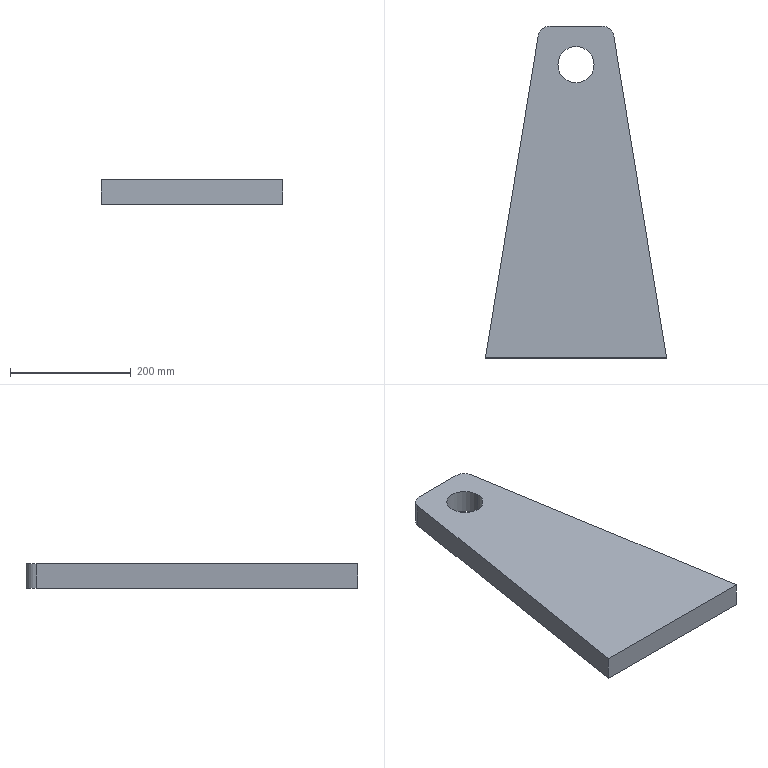Part | SolidWorks | features Extrusion 1 | 1 solid | 10 faces | box 300 x 550 x 40 mm | volume 4502251 mm3 | plane 6 | cylinder 4 | commonest cylinder face diameters 40 x2 60 x2
STEP:
#1=CARTESIAN_POINT('',(120.,486.,40.));
#2=VERTEX_POINT('',#1);
#3=CARTESIAN_POINT('',(180.,486.,40.));
#4=VERTEX_POINT('',#3);
#5=CARTESIAN_POINT('',(150.,486.,40.));
#6=DIRECTION('',(0.,0.,1.));
#7=DIRECTION('',(1.,0.,0.));
#8=AXIS2_PLACEMENT_3D('',#5,#6,#7);
#9=CIRCLE('',#8,30.);
#10=EDGE_CURVE('',#2,#4,#9,.T.);
#11=ORIENTED_EDGE('',*,*,#10,.T.);
#12=CARTESIAN_POINT('',(180.,486.,0.));
#13=VERTEX_POINT('',#12);
#14=CARTESIAN_POINT('',(180.,486.,40.));
#15=DIRECTION('',(0.,0.,-1.));
#16=VECTOR('',#15,1000.);
#17=LINE('',#14,#16);
#18=EDGE_CURVE('',#4,#13,#17,.T.);
#19=ORIENTED_EDGE('',*,*,#18,.T.);
#20=CARTESIAN_POINT('',(120.,486.,0.));
#21=VERTEX_POINT('',#20);
#22=CARTESIAN_POINT('',(150.,486.,0.));
#23=DIRECTION('',(0.,0.,1.));
#24=DIRECTION('',(1.,0.,0.));
#25=AXIS2_PLACEMENT_3D('',#22,#23,#24);
#26=CIRCLE('',#25,30.);
#27=EDGE_CURVE('',#21,#13,#26,.T.);
#28=ORIENTED_EDGE('',*,*,#27,.F.);
#29=CARTESIAN_POINT('',(120.,486.,40.));
#30=DIRECTION('',(0.,0.,-1.));
#31=VECTOR('',#30,1000.);
#32=LINE('',#29,#31);
#33=EDGE_CURVE('',#2,#21,#32,.T.);
#34=ORIENTED_EDGE('',*,*,#33,.F.);
#35=EDGE_LOOP('',(#11,#19,#28,#34));
#36=FACE_OUTER_BOUND('',#35,.T.);
#37=CARTESIAN_POINT('',(150.,486.,40.));
#38=DIRECTION('',(0.,0.,-1.));
#39=DIRECTION('',(-1.,0.,0.));
#40=AXIS2_PLACEMENT_3D('',#37,#38,#39);
#41=CYLINDRICAL_SURFACE('',#40,30.);
#42=ADVANCED_FACE('',(#36),#41,.F.);
#43=CARTESIAN_POINT('',(87.256,533.23,40.));
#44=VERTEX_POINT('',#43);
#45=CARTESIAN_POINT('',(0.,0.,40.));
#46=VERTEX_POINT('',#45);
#47=CARTESIAN_POINT('',(0.,0.,40.));
#48=DIRECTION('',(-0.1615,-0.9869,0.));
#49=VECTOR('',#48,1000.);
#50=LINE('',#47,#49);
#51=EDGE_CURVE('',#44,#46,#50,.T.);
#52=ORIENTED_EDGE('',*,*,#51,.T.);
#53=CARTESIAN_POINT('',(300.,0.,40.));
#54=VERTEX_POINT('',#53);
#55=CARTESIAN_POINT('',(0.,0.,40.));
#56=DIRECTION('',(1.,0.,0.));
#57=VECTOR('',#56,1000.);
#58=LINE('',#55,#57);
#59=EDGE_CURVE('',#46,#54,#58,.T.);
#60=ORIENTED_EDGE('',*,*,#59,.T.);
#61=CARTESIAN_POINT('',(212.744,533.23,40.));
#62=VERTEX_POINT('',#61);
#63=CARTESIAN_POINT('',(300.,0.,40.));
#64=DIRECTION('',(-0.1615,0.9869,0.));
#65=VECTOR('',#64,1000.);
#66=LINE('',#63,#65);
#67=EDGE_CURVE('',#54,#62,#66,.T.);
#68=ORIENTED_EDGE('',*,*,#67,.T.);
#69=CARTESIAN_POINT('',(193.007,550.,40.));
#70=VERTEX_POINT('',#69);
#71=CARTESIAN_POINT('',(193.007,530.,40.));
#72=DIRECTION('',(0.,0.,1.));
#73=DIRECTION('',(-1.,0.,0.));
#74=AXIS2_PLACEMENT_3D('',#71,#72,#73);
#75=CIRCLE('',#74,20.);
#76=EDGE_CURVE('',#62,#70,#75,.T.);
#77=ORIENTED_EDGE('',*,*,#76,.T.);
#78=CARTESIAN_POINT('',(106.993,550.,40.));
#79=VERTEX_POINT('',#78);
#80=CARTESIAN_POINT('',(106.993,550.,40.));
#81=DIRECTION('',(-1.,0.,0.));
#82=VECTOR('',#81,1000.);
#83=LINE('',#80,#82);
#84=EDGE_CURVE('',#70,#79,#83,.T.);
#85=ORIENTED_EDGE('',*,*,#84,.T.);
#86=CARTESIAN_POINT('',(106.993,530.,40.));
#87=DIRECTION('',(0.,0.,1.));
#88=DIRECTION('',(-1.,0.,0.));
#89=AXIS2_PLACEMENT_3D('',#86,#87,#88);
#90=CIRCLE('',#89,20.);
#91=EDGE_CURVE('',#79,#44,#90,.T.);
#92=ORIENTED_EDGE('',*,*,#91,.T.);
#93=EDGE_LOOP('',(#52,#60,#68,#77,#85,#92));
#94=FACE_OUTER_BOUND('',#93,.T.);
#95=ORIENTED_EDGE('',*,*,#10,.F.);
#96=CARTESIAN_POINT('',(150.,486.,40.));
#97=DIRECTION('',(0.,0.,1.));
#98=DIRECTION('',(1.,0.,0.));
#99=AXIS2_PLACEMENT_3D('',#96,#97,#98);
#100=CIRCLE('',#99,30.);
#101=EDGE_CURVE('',#4,#2,#100,.T.);
#102=ORIENTED_EDGE('',*,*,#101,.F.);
#103=EDGE_LOOP('',(#95,#102));
#104=FACE_BOUND('',#103,.T.);
#105=CARTESIAN_POINT('',(106.993,530.,40.));
#106=DIRECTION('',(0.,0.,-1.));
#107=DIRECTION('',(-1.,0.,0.));
#108=AXIS2_PLACEMENT_3D('',#105,#106,#107);
#109=PLANE('',#108);
#110=ADVANCED_FACE('',(#94,#104),#109,.F.);
#111=CARTESIAN_POINT('',(87.256,533.23,0.));
#112=VERTEX_POINT('',#111);
#113=CARTESIAN_POINT('',(0.,0.,0.));
#114=VERTEX_POINT('',#113);
#115=CARTESIAN_POINT('',(0.,0.,0.));
#116=DIRECTION('',(-0.1615,-0.9869,0.));
#117=VECTOR('',#116,1000.);
#118=LINE('',#115,#117);
#119=EDGE_CURVE('',#112,#114,#118,.T.);
#120=ORIENTED_EDGE('',*,*,#119,.F.);
#121=CARTESIAN_POINT('',(106.993,550.,0.));
#122=VERTEX_POINT('',#121);
#123=CARTESIAN_POINT('',(106.993,530.,0.));
#124=DIRECTION('',(0.,0.,1.));
#125=DIRECTION('',(-1.,0.,0.));
#126=AXIS2_PLACEMENT_3D('',#123,#124,#125);
#127=CIRCLE('',#126,20.);
#128=EDGE_CURVE('',#122,#112,#127,.T.);
#129=ORIENTED_EDGE('',*,*,#128,.F.);
#130=CARTESIAN_POINT('',(193.007,550.,0.));
#131=VERTEX_POINT('',#130);
#132=CARTESIAN_POINT('',(106.993,550.,0.));
#133=DIRECTION('',(-1.,0.,0.));
#134=VECTOR('',#133,1000.);
#135=LINE('',#132,#134);
#136=EDGE_CURVE('',#131,#122,#135,.T.);
#137=ORIENTED_EDGE('',*,*,#136,.F.);
#138=CARTESIAN_POINT('',(212.744,533.23,0.));
#139=VERTEX_POINT('',#138);
#140=CARTESIAN_POINT('',(193.007,530.,0.));
#141=DIRECTION('',(0.,0.,1.));
#142=DIRECTION('',(-1.,0.,0.));
#143=AXIS2_PLACEMENT_3D('',#140,#141,#142);
#144=CIRCLE('',#143,20.);
#145=EDGE_CURVE('',#139,#131,#144,.T.);
#146=ORIENTED_EDGE('',*,*,#145,.F.);
#147=CARTESIAN_POINT('',(300.,0.,0.));
#148=VERTEX_POINT('',#147);
#149=CARTESIAN_POINT('',(300.,0.,0.));
#150=DIRECTION('',(-0.1615,0.9869,0.));
#151=VECTOR('',#150,1000.);
#152=LINE('',#149,#151);
#153=EDGE_CURVE('',#148,#139,#152,.T.);
#154=ORIENTED_EDGE('',*,*,#153,.F.);
#155=CARTESIAN_POINT('',(0.,0.,0.));
#156=DIRECTION('',(1.,0.,0.));
#157=VECTOR('',#156,1000.);
#158=LINE('',#155,#157);
#159=EDGE_CURVE('',#114,#148,#158,.T.);
#160=ORIENTED_EDGE('',*,*,#159,.F.);
#161=EDGE_LOOP('',(#120,#129,#137,#146,#154,#160));
#162=FACE_OUTER_BOUND('',#161,.T.);
#163=ORIENTED_EDGE('',*,*,#27,.T.);
#164=CARTESIAN_POINT('',(150.,486.,0.));
#165=DIRECTION('',(0.,0.,1.));
#166=DIRECTION('',(1.,0.,0.));
#167=AXIS2_PLACEMENT_3D('',#164,#165,#166);
#168=CIRCLE('',#167,30.);
#169=EDGE_CURVE('',#13,#21,#168,.T.);
#170=ORIENTED_EDGE('',*,*,#169,.T.);
#171=EDGE_LOOP('',(#163,#170));
#172=FACE_BOUND('',#171,.T.);
#173=CARTESIAN_POINT('',(106.993,530.,0.));
#174=DIRECTION('',(0.,0.,-1.));
#175=DIRECTION('',(-1.,0.,0.));
#176=AXIS2_PLACEMENT_3D('',#173,#174,#175);
#177=PLANE('',#176);
#178=ADVANCED_FACE('',(#162,#172),#177,.T.);
#179=ORIENTED_EDGE('',*,*,#119,.T.);
#180=CARTESIAN_POINT('',(0.,0.,40.));
#181=DIRECTION('',(0.,0.,-1.));
#182=VECTOR('',#181,1000.);
#183=LINE('',#180,#182);
#184=EDGE_CURVE('',#46,#114,#183,.T.);
#185=ORIENTED_EDGE('',*,*,#184,.F.);
#186=ORIENTED_EDGE('',*,*,#51,.F.);
#187=CARTESIAN_POINT('',(87.256,533.23,40.));
#188=DIRECTION('',(0.,0.,-1.));
#189=VECTOR('',#188,1000.);
#190=LINE('',#187,#189);
#191=EDGE_CURVE('',#44,#112,#190,.T.);
#192=ORIENTED_EDGE('',*,*,#191,.T.);
#193=EDGE_LOOP('',(#179,#185,#186,#192));
#194=FACE_OUTER_BOUND('',#193,.T.);
#195=CARTESIAN_POINT('',(0.,0.,40.));
#196=DIRECTION('',(0.9869,-0.1615,0.));
#197=DIRECTION('',(0.1615,0.9869,0.));
#198=AXIS2_PLACEMENT_3D('',#195,#196,#197);
#199=PLANE('',#198);
#200=ADVANCED_FACE('',(#194),#199,.F.);
#201=ORIENTED_EDGE('',*,*,#159,.T.);
#202=CARTESIAN_POINT('',(300.,0.,40.));
#203=DIRECTION('',(0.,0.,-1.));
#204=VECTOR('',#203,1000.);
#205=LINE('',#202,#204);
#206=EDGE_CURVE('',#54,#148,#205,.T.);
#207=ORIENTED_EDGE('',*,*,#206,.F.);
#208=ORIENTED_EDGE('',*,*,#59,.F.);
#209=ORIENTED_EDGE('',*,*,#184,.T.);
#210=EDGE_LOOP('',(#201,#207,#208,#209));
#211=FACE_OUTER_BOUND('',#210,.T.);
#212=CARTESIAN_POINT('',(0.,0.,40.));
#213=DIRECTION('',(0.,1.,0.));
#214=DIRECTION('',(0.,0.,1.));
#215=AXIS2_PLACEMENT_3D('',#212,#213,#214);
#216=PLANE('',#215);
#217=ADVANCED_FACE('',(#211),#216,.F.);
#218=ORIENTED_EDGE('',*,*,#153,.T.);
#219=CARTESIAN_POINT('',(212.744,533.23,40.));
#220=DIRECTION('',(0.,0.,-1.));
#221=VECTOR('',#220,1000.);
#222=LINE('',#219,#221);
#223=EDGE_CURVE('',#62,#139,#222,.T.);
#224=ORIENTED_EDGE('',*,*,#223,.F.);
#225=ORIENTED_EDGE('',*,*,#67,.F.);
#226=ORIENTED_EDGE('',*,*,#206,.T.);
#227=EDGE_LOOP('',(#218,#224,#225,#226));
#228=FACE_OUTER_BOUND('',#227,.T.);
#229=CARTESIAN_POINT('',(300.,0.,40.));
#230=DIRECTION('',(-0.9869,-0.1615,0.));
#231=DIRECTION('',(0.1615,-0.9869,0.));
#232=AXIS2_PLACEMENT_3D('',#229,#230,#231);
#233=PLANE('',#232);
#234=ADVANCED_FACE('',(#228),#233,.F.);
#235=ORIENTED_EDGE('',*,*,#145,.T.);
#236=CARTESIAN_POINT('',(193.007,550.,40.));
#237=DIRECTION('',(0.,0.,-1.));
#238=VECTOR('',#237,1000.);
#239=LINE('',#236,#238);
#240=EDGE_CURVE('',#70,#131,#239,.T.);
#241=ORIENTED_EDGE('',*,*,#240,.F.);
#242=ORIENTED_EDGE('',*,*,#76,.F.);
#243=ORIENTED_EDGE('',*,*,#223,.T.);
#244=EDGE_LOOP('',(#235,#241,#242,#243));
#245=FACE_OUTER_BOUND('',#244,.T.);
#246=CARTESIAN_POINT('',(193.007,530.,40.));
#247=DIRECTION('',(0.,0.,-1.));
#248=DIRECTION('',(-1.,0.,0.));
#249=AXIS2_PLACEMENT_3D('',#246,#247,#248);
#250=CYLINDRICAL_SURFACE('',#249,20.);
#251=ADVANCED_FACE('',(#245),#250,.T.);
#252=ORIENTED_EDGE('',*,*,#136,.T.);
#253=CARTESIAN_POINT('',(106.993,550.,40.));
#254=DIRECTION('',(0.,0.,-1.));
#255=VECTOR('',#254,1000.);
#256=LINE('',#253,#255);
#257=EDGE_CURVE('',#79,#122,#256,.T.);
#258=ORIENTED_EDGE('',*,*,#257,.F.);
#259=ORIENTED_EDGE('',*,*,#84,.F.);
#260=ORIENTED_EDGE('',*,*,#240,.T.);
#261=EDGE_LOOP('',(#252,#258,#259,#260));
#262=FACE_OUTER_BOUND('',#261,.T.);
#263=CARTESIAN_POINT('',(106.993,550.,40.));
#264=DIRECTION('',(0.,-1.,0.));
#265=DIRECTION('',(1.,0.,0.));
#266=AXIS2_PLACEMENT_3D('',#263,#264,#265);
#267=PLANE('',#266);
#268=ADVANCED_FACE('',(#262),#267,.F.);
#269=ORIENTED_EDGE('',*,*,#128,.T.);
#270=ORIENTED_EDGE('',*,*,#191,.F.);
#271=ORIENTED_EDGE('',*,*,#91,.F.);
#272=ORIENTED_EDGE('',*,*,#257,.T.);
#273=EDGE_LOOP('',(#269,#270,#271,#272));
#274=FACE_OUTER_BOUND('',#273,.T.);
#275=CARTESIAN_POINT('',(106.993,530.,40.));
#276=DIRECTION('',(0.,0.,-1.));
#277=DIRECTION('',(-1.,0.,0.));
#278=AXIS2_PLACEMENT_3D('',#275,#276,#277);
#279=CYLINDRICAL_SURFACE('',#278,20.);
#280=ADVANCED_FACE('',(#274),#279,.T.);
#281=ORIENTED_EDGE('',*,*,#18,.F.);
#282=ORIENTED_EDGE('',*,*,#101,.T.);
#283=ORIENTED_EDGE('',*,*,#33,.T.);
#284=ORIENTED_EDGE('',*,*,#169,.F.);
#285=EDGE_LOOP('',(#281,#282,#283,#284));
#286=FACE_OUTER_BOUND('',#285,.T.);
#287=CARTESIAN_POINT('',(150.,486.,40.));
#288=DIRECTION('',(0.,0.,-1.));
#289=DIRECTION('',(-1.,0.,0.));
#290=AXIS2_PLACEMENT_3D('',#287,#288,#289);
#291=CYLINDRICAL_SURFACE('',#290,30.);
#292=ADVANCED_FACE('',(#286),#291,.F.);
#293=CLOSED_SHELL('',(#42,#110,#178,#200,#217,#234,#251,#268,#280,#292));
#294=MANIFOLD_SOLID_BREP('',#293);
#295=CARTESIAN_POINT('',(0.,0.,0.));
#296=DIRECTION('',(0.,0.,1.));
#297=DIRECTION('',(1.,0.,0.));
#298=AXIS2_PLACEMENT_3D('',#295,#296,#297);
#299=(LENGTH_UNIT()NAMED_UNIT(*)SI_UNIT(.MILLI.,.METRE.));
#300=UNCERTAINTY_MEASURE_WITH_UNIT(LENGTH_MEASURE(0.00001),#299,'','');
#301=(NAMED_UNIT(*)PLANE_ANGLE_UNIT()SI_UNIT($,.RADIAN.));
#302=(NAMED_UNIT(*)SI_UNIT($,.STERADIAN.)SOLID_ANGLE_UNIT());
#303=(GEOMETRIC_REPRESENTATION_CONTEXT(3)GLOBAL_UNCERTAINTY_ASSIGNED_CONTEXT((#300))GLOBAL_UNIT_ASSIGNED_CONTEXT((#299,#301,#302))REPRESENTATION_CONTEXT('',''));
#304=ADVANCED_BREP_SHAPE_REPRESENTATION('',(#294,#298),#303);